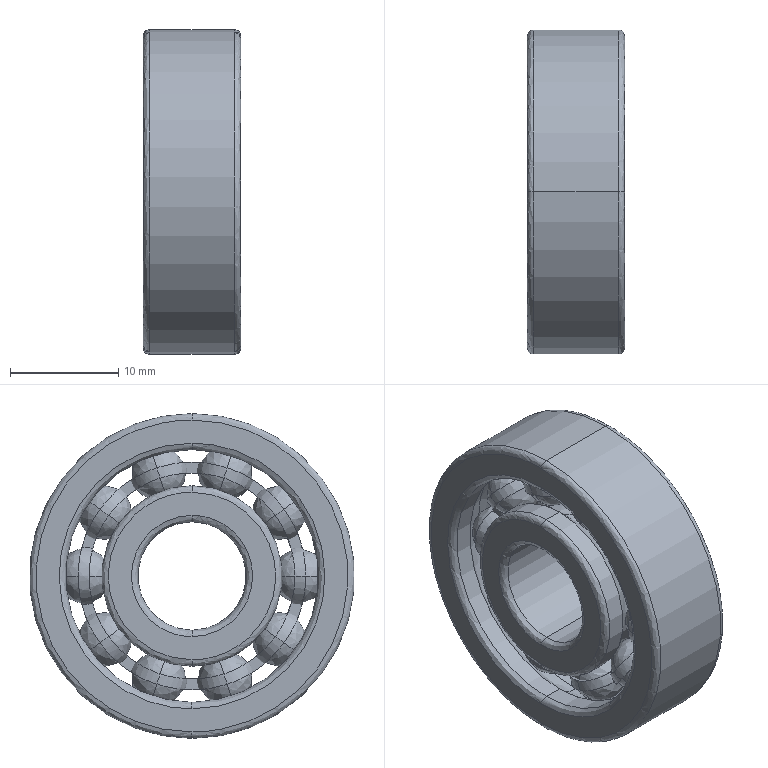Part | SolidWorks | features BaseBody 12 | 12 solids | 139 faces | box 9 x 30 x 30 mm | volume 4206 mm3 | spline 65 | cylinder 50 | plane 24 | commonest cylinder face diameters 19 x19 21 x19 16.667 x4 23.333 x4 10 x2 30 x2